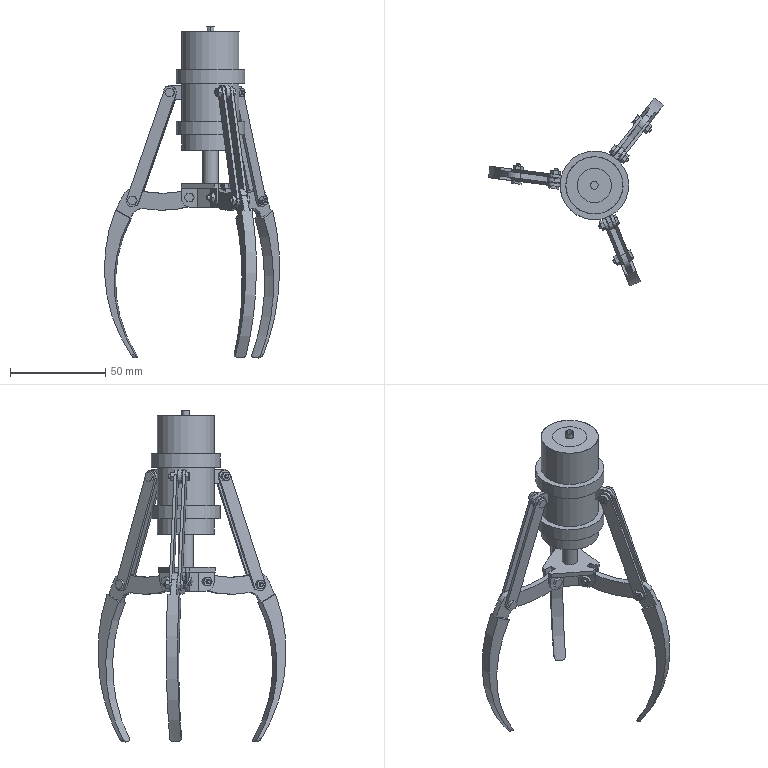Part | NX | features BREP 26, DATUM_CSYS 26, EXTRUDE 23, SKETCH 21, CPROJ 8, EXTRACT_STRING 6, BLEND 4, HOLE PACKAGE 3, SIMPLE HOLE 3, UNITE 3, DATUM_PLANE 2, EXTRACT_BODY 2, Instance Feature 2, Delete Body 1, LINKED_FACE 1, Pattern Feature 1, Pattern Geometry 1, SHELL 1 | 32 solids | 524 faces | box 91.731 x 98.46 x 173.883 mm | volume 50064 mm3 | plane 270 | cone 135 | cylinder 110 | torus 9 | commonest cylinder face diameters 2 x45 4 x14 6.5 x12 10 x6 7.5 x3 10.7 x3